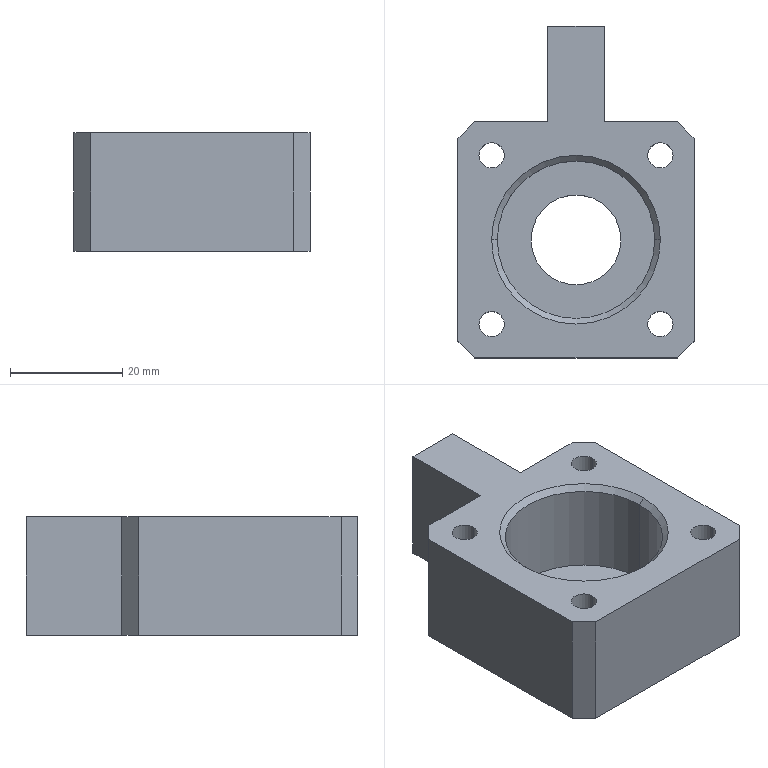Part | SolidWorks | features ICE 4, Chamfer 2, HoleWzd 2, Extrusion 1 | 1 solid | 49 faces | box 42 x 59 x 21 mm | volume 26880 mm3 | cylinder 24 | plane 19 | cone 6 | commonest cylinder face diameters 4.5 x8 8 x8 2.5 x4 16 x2 28 x2
STEP:
#1=CARTESIAN_POINT('',(-14.,23.25,20.));
#2=VERTEX_POINT('',#1);
#3=CARTESIAN_POINT('',(14.,23.25,20.));
#4=VERTEX_POINT('',#3);
#5=CARTESIAN_POINT('',(0.,23.25,20.));
#6=DIRECTION('',(0.,0.,1.));
#7=DIRECTION('',(1.,0.,0.));
#8=AXIS2_PLACEMENT_3D('',#5,#6,#7);
#9=CIRCLE('',#8,14.);
#10=EDGE_CURVE('',#2,#4,#9,.T.);
#11=ORIENTED_EDGE('',*,*,#10,.F.);
#12=CARTESIAN_POINT('',(-15.,23.25,21.));
#13=VERTEX_POINT('',#12);
#14=CARTESIAN_POINT('',(-14.,23.25,20.));
#15=DIRECTION('',(-0.7071,0.,0.7071));
#16=VECTOR('',#15,1000.);
#17=LINE('',#14,#16);
#18=EDGE_CURVE('',#2,#13,#17,.T.);
#19=ORIENTED_EDGE('',*,*,#18,.T.);
#20=CARTESIAN_POINT('',(15.,23.25,21.));
#21=VERTEX_POINT('',#20);
#22=CARTESIAN_POINT('',(0.,23.25,21.));
#23=DIRECTION('',(0.,0.,-1.));
#24=DIRECTION('',(1.,0.,0.));
#25=AXIS2_PLACEMENT_3D('',#22,#23,#24);
#26=CIRCLE('',#25,15.);
#27=EDGE_CURVE('',#21,#13,#26,.T.);
#28=ORIENTED_EDGE('',*,*,#27,.F.);
#29=CARTESIAN_POINT('',(14.,23.25,20.));
#30=DIRECTION('',(0.7071,0.,0.7071));
#31=VECTOR('',#30,1000.);
#32=LINE('',#29,#31);
#33=EDGE_CURVE('',#4,#21,#32,.T.);
#34=ORIENTED_EDGE('',*,*,#33,.F.);
#35=EDGE_LOOP('',(#11,#19,#28,#34));
#36=FACE_OUTER_BOUND('',#35,.T.);
#37=CARTESIAN_POINT('',(0.,23.25,20.));
#38=DIRECTION('',(0.,0.,1.));
#39=DIRECTION('',(1.,0.,0.));
#40=AXIS2_PLACEMENT_3D('',#37,#38,#39);
#41=CONICAL_SURFACE('',#40,14.,0.7854);
#42=ADVANCED_FACE('',(#36),#41,.F.);
#43=CARTESIAN_POINT('',(1.25,57.75,7.));
#44=VERTEX_POINT('',#43);
#45=CARTESIAN_POINT('',(-1.25,57.75,7.));
#46=VERTEX_POINT('',#45);
#47=CARTESIAN_POINT('',(0.,57.75,7.));
#48=DIRECTION('',(0.,0.,-1.));
#49=DIRECTION('',(-1.,0.,0.));
#50=AXIS2_PLACEMENT_3D('',#47,#48,#49);
#51=CIRCLE('',#50,1.25);
#52=EDGE_CURVE('',#44,#46,#51,.T.);
#53=ORIENTED_EDGE('',*,*,#52,.F.);
#54=CARTESIAN_POINT('',(1.25,57.75,0.));
#55=VERTEX_POINT('',#54);
#56=CARTESIAN_POINT('',(1.25,57.75,0.));
#57=DIRECTION('',(0.,0.,-1.));
#58=VECTOR('',#57,1000.);
#59=LINE('',#56,#58);
#60=EDGE_CURVE('',#44,#55,#59,.T.);
#61=ORIENTED_EDGE('',*,*,#60,.T.);
#62=CARTESIAN_POINT('',(-1.25,57.75,0.));
#63=VERTEX_POINT('',#62);
#64=CARTESIAN_POINT('',(0.,57.75,0.));
#65=DIRECTION('',(0.,0.,-1.));
#66=DIRECTION('',(-1.,0.,0.));
#67=AXIS2_PLACEMENT_3D('',#64,#65,#66);
#68=CIRCLE('',#67,1.25);
#69=EDGE_CURVE('',#55,#63,#68,.T.);
#70=ORIENTED_EDGE('',*,*,#69,.T.);
#71=CARTESIAN_POINT('',(-1.25,57.75,0.));
#72=DIRECTION('',(0.,0.,-1.));
#73=VECTOR('',#72,1000.);
#74=LINE('',#71,#73);
#75=EDGE_CURVE('',#46,#63,#74,.T.);
#76=ORIENTED_EDGE('',*,*,#75,.F.);
#77=EDGE_LOOP('',(#53,#61,#70,#76));
#78=FACE_OUTER_BOUND('',#77,.T.);
#79=CARTESIAN_POINT('',(0.,57.75,0.));
#80=DIRECTION('',(0.,0.,-1.));
#81=DIRECTION('',(-1.,0.,0.));
#82=AXIS2_PLACEMENT_3D('',#79,#80,#81);
#83=CYLINDRICAL_SURFACE('',#82,1.25);
#84=ADVANCED_FACE('',(#78),#83,.F.);
#85=CARTESIAN_POINT('',(0.,57.75,7.751));
#86=VERTEX_POINT('',#85);
#87=CARTESIAN_POINT('',(-1.25,57.75,7.));
#88=DIRECTION('',(-0.8572,0.,-0.515));
#89=VECTOR('',#88,1000.);
#90=LINE('',#87,#89);
#91=EDGE_CURVE('',#86,#46,#90,.T.);
#92=ORIENTED_EDGE('',*,*,#91,.F.);
#93=CARTESIAN_POINT('',(1.25,57.75,7.));
#94=DIRECTION('',(0.8572,0.,-0.515));
#95=VECTOR('',#94,1000.);
#96=LINE('',#93,#95);
#97=EDGE_CURVE('',#86,#44,#96,.T.);
#98=ORIENTED_EDGE('',*,*,#97,.T.);
#99=ORIENTED_EDGE('',*,*,#52,.T.);
#100=EDGE_LOOP('',(#92,#98,#99));
#101=FACE_OUTER_BOUND('',#100,.T.);
#102=CARTESIAN_POINT('',(0.,57.75,7.));
#103=DIRECTION('',(0.,0.,-1.));
#104=DIRECTION('',(-1.,0.,0.));
#105=AXIS2_PLACEMENT_3D('',#102,#103,#104);
#106=CONICAL_SURFACE('',#105,1.25,1.03);
#107=ADVANCED_FACE('',(#101),#106,.F.);
#108=CARTESIAN_POINT('',(1.25,39.25,7.));
#109=VERTEX_POINT('',#108);
#110=CARTESIAN_POINT('',(-1.25,39.25,7.));
#111=VERTEX_POINT('',#110);
#112=CARTESIAN_POINT('',(0.,39.25,7.));
#113=DIRECTION('',(0.,0.,-1.));
#114=DIRECTION('',(-1.,0.,0.));
#115=AXIS2_PLACEMENT_3D('',#112,#113,#114);
#116=CIRCLE('',#115,1.25);
#117=EDGE_CURVE('',#109,#111,#116,.T.);
#118=ORIENTED_EDGE('',*,*,#117,.F.);
#119=CARTESIAN_POINT('',(1.25,39.25,0.));
#120=VERTEX_POINT('',#119);
#121=CARTESIAN_POINT('',(1.25,39.25,0.));
#122=DIRECTION('',(0.,0.,-1.));
#123=VECTOR('',#122,1000.);
#124=LINE('',#121,#123);
#125=EDGE_CURVE('',#109,#120,#124,.T.);
#126=ORIENTED_EDGE('',*,*,#125,.T.);
#127=CARTESIAN_POINT('',(-1.25,39.25,0.));
#128=VERTEX_POINT('',#127);
#129=CARTESIAN_POINT('',(0.,39.25,0.));
#130=DIRECTION('',(0.,0.,-1.));
#131=DIRECTION('',(-1.,0.,0.));
#132=AXIS2_PLACEMENT_3D('',#129,#130,#131);
#133=CIRCLE('',#132,1.25);
#134=EDGE_CURVE('',#120,#128,#133,.T.);
#135=ORIENTED_EDGE('',*,*,#134,.T.);
#136=CARTESIAN_POINT('',(-1.25,39.25,0.));
#137=DIRECTION('',(0.,0.,-1.));
#138=VECTOR('',#137,1000.);
#139=LINE('',#136,#138);
#140=EDGE_CURVE('',#111,#128,#139,.T.);
#141=ORIENTED_EDGE('',*,*,#140,.F.);
#142=EDGE_LOOP('',(#118,#126,#135,#141));
#143=FACE_OUTER_BOUND('',#142,.T.);
#144=CARTESIAN_POINT('',(0.,39.25,0.));
#145=DIRECTION('',(0.,0.,-1.));
#146=DIRECTION('',(-1.,0.,0.));
#147=AXIS2_PLACEMENT_3D('',#144,#145,#146);
#148=CYLINDRICAL_SURFACE('',#147,1.25);
#149=ADVANCED_FACE('',(#143),#148,.F.);
#150=CARTESIAN_POINT('',(0.,39.25,7.751));
#151=VERTEX_POINT('',#150);
#152=CARTESIAN_POINT('',(-1.25,39.25,7.));
#153=DIRECTION('',(-0.8572,0.,-0.515));
#154=VECTOR('',#153,1000.);
#155=LINE('',#152,#154);
#156=EDGE_CURVE('',#151,#111,#155,.T.);
#157=ORIENTED_EDGE('',*,*,#156,.F.);
#158=CARTESIAN_POINT('',(1.25,39.25,7.));
#159=DIRECTION('',(0.8572,0.,-0.515));
#160=VECTOR('',#159,1000.);
#161=LINE('',#158,#160);
#162=EDGE_CURVE('',#151,#109,#161,.T.);
#163=ORIENTED_EDGE('',*,*,#162,.T.);
#164=ORIENTED_EDGE('',*,*,#117,.T.);
#165=EDGE_LOOP('',(#157,#163,#164));
#166=FACE_OUTER_BOUND('',#165,.T.);
#167=CARTESIAN_POINT('',(0.,39.25,7.));
#168=DIRECTION('',(0.,0.,-1.));
#169=DIRECTION('',(-1.,0.,0.));
#170=AXIS2_PLACEMENT_3D('',#167,#168,#169);
#171=CONICAL_SURFACE('',#170,1.25,1.03);
#172=ADVANCED_FACE('',(#166),#171,.F.);
#173=CARTESIAN_POINT('',(19.,38.25,4.6));
#174=VERTEX_POINT('',#173);
#175=CARTESIAN_POINT('',(11.,38.25,4.6));
#176=VERTEX_POINT('',#175);
#177=CARTESIAN_POINT('',(15.,38.25,4.6));
#178=DIRECTION('',(0.,0.,-1.));
#179=DIRECTION('',(-1.,0.,0.));
#180=AXIS2_PLACEMENT_3D('',#177,#178,#179);
#181=CIRCLE('',#180,4.);
#182=EDGE_CURVE('',#174,#176,#181,.T.);
#183=ORIENTED_EDGE('',*,*,#182,.F.);
#184=CARTESIAN_POINT('',(19.,38.25,0.));
#185=VERTEX_POINT('',#184);
#186=CARTESIAN_POINT('',(19.,38.25,0.));
#187=DIRECTION('',(0.,0.,-1.));
#188=VECTOR('',#187,1000.);
#189=LINE('',#186,#188);
#190=EDGE_CURVE('',#174,#185,#189,.T.);
#191=ORIENTED_EDGE('',*,*,#190,.T.);
#192=CARTESIAN_POINT('',(11.,38.25,0.));
#193=VERTEX_POINT('',#192);
#194=CARTESIAN_POINT('',(15.,38.25,0.));
#195=DIRECTION('',(0.,0.,-1.));
#196=DIRECTION('',(-1.,0.,0.));
#197=AXIS2_PLACEMENT_3D('',#194,#195,#196);
#198=CIRCLE('',#197,4.);
#199=EDGE_CURVE('',#185,#193,#198,.T.);
#200=ORIENTED_EDGE('',*,*,#199,.T.);
#201=CARTESIAN_POINT('',(11.,38.25,0.));
#202=DIRECTION('',(0.,0.,-1.));
#203=VECTOR('',#202,1000.);
#204=LINE('',#201,#203);
#205=EDGE_CURVE('',#176,#193,#204,.T.);
#206=ORIENTED_EDGE('',*,*,#205,.F.);
#207=EDGE_LOOP('',(#183,#191,#200,#206));
#208=FACE_OUTER_BOUND('',#207,.T.);
#209=CARTESIAN_POINT('',(15.,38.25,0.));
#210=DIRECTION('',(0.,0.,-1.));
#211=DIRECTION('',(-1.,0.,0.));
#212=AXIS2_PLACEMENT_3D('',#209,#210,#211);
#213=CYLINDRICAL_SURFACE('',#212,4.);
#214=ADVANCED_FACE('',(#208),#213,.F.);
#215=CARTESIAN_POINT('',(12.75,38.25,21.));
#216=VERTEX_POINT('',#215);
#217=CARTESIAN_POINT('',(17.25,38.25,21.));
#218=VERTEX_POINT('',#217);
#219=CARTESIAN_POINT('',(15.,38.25,21.));
#220=DIRECTION('',(0.,0.,1.));
#221=DIRECTION('',(1.,0.,0.));
#222=AXIS2_PLACEMENT_3D('',#219,#220,#221);
#223=CIRCLE('',#222,2.25);
#224=EDGE_CURVE('',#216,#218,#223,.T.);
#225=ORIENTED_EDGE('',*,*,#224,.T.);
#226=CARTESIAN_POINT('',(17.25,38.25,4.6));
#227=VERTEX_POINT('',#226);
#228=CARTESIAN_POINT('',(17.25,38.25,0.));
#229=DIRECTION('',(0.,0.,-1.));
#230=VECTOR('',#229,1000.);
#231=LINE('',#228,#230);
#232=EDGE_CURVE('',#218,#227,#231,.T.);
#233=ORIENTED_EDGE('',*,*,#232,.T.);
#234=CARTESIAN_POINT('',(12.75,38.25,4.6));
#235=VERTEX_POINT('',#234);
#236=CARTESIAN_POINT('',(15.,38.25,4.6));
#237=DIRECTION('',(0.,0.,-1.));
#238=DIRECTION('',(-1.,0.,0.));
#239=AXIS2_PLACEMENT_3D('',#236,#237,#238);
#240=CIRCLE('',#239,2.25);
#241=EDGE_CURVE('',#227,#235,#240,.T.);
#242=ORIENTED_EDGE('',*,*,#241,.T.);
#243=CARTESIAN_POINT('',(12.75,38.25,0.));
#244=DIRECTION('',(0.,0.,-1.));
#245=VECTOR('',#244,1000.);
#246=LINE('',#243,#245);
#247=EDGE_CURVE('',#216,#235,#246,.T.);
#248=ORIENTED_EDGE('',*,*,#247,.F.);
#249=EDGE_LOOP('',(#225,#233,#242,#248));
#250=FACE_OUTER_BOUND('',#249,.T.);
#251=CARTESIAN_POINT('',(15.,38.25,0.));
#252=DIRECTION('',(0.,0.,-1.));
#253=DIRECTION('',(-1.,0.,0.));
#254=AXIS2_PLACEMENT_3D('',#251,#252,#253);
#255=CYLINDRICAL_SURFACE('',#254,2.25);
#256=ADVANCED_FACE('',(#250),#255,.F.);
#257=CARTESIAN_POINT('',(-11.,38.25,4.6));
#258=VERTEX_POINT('',#257);
#259=CARTESIAN_POINT('',(-19.,38.25,4.6));
#260=VERTEX_POINT('',#259);
#261=CARTESIAN_POINT('',(-15.,38.25,4.6));
#262=DIRECTION('',(0.,0.,-1.));
#263=DIRECTION('',(-1.,0.,0.));
#264=AXIS2_PLACEMENT_3D('',#261,#262,#263);
#265=CIRCLE('',#264,4.);
#266=EDGE_CURVE('',#258,#260,#265,.T.);
#267=ORIENTED_EDGE('',*,*,#266,.F.);
#268=CARTESIAN_POINT('',(-11.,38.25,0.));
#269=VERTEX_POINT('',#268);
#270=CARTESIAN_POINT('',(-11.,38.25,0.));
#271=DIRECTION('',(0.,0.,-1.));
#272=VECTOR('',#271,1000.);
#273=LINE('',#270,#272);
#274=EDGE_CURVE('',#258,#269,#273,.T.);
#275=ORIENTED_EDGE('',*,*,#274,.T.);
#276=CARTESIAN_POINT('',(-19.,38.25,0.));
#277=VERTEX_POINT('',#276);
#278=CARTESIAN_POINT('',(-15.,38.25,0.));
#279=DIRECTION('',(0.,0.,-1.));
#280=DIRECTION('',(-1.,0.,0.));
#281=AXIS2_PLACEMENT_3D('',#278,#279,#280);
#282=CIRCLE('',#281,4.);
#283=EDGE_CURVE('',#269,#277,#282,.T.);
#284=ORIENTED_EDGE('',*,*,#283,.T.);
#285=CARTESIAN_POINT('',(-19.,38.25,0.));
#286=DIRECTION('',(0.,0.,-1.));
#287=VECTOR('',#286,1000.);
#288=LINE('',#285,#287);
#289=EDGE_CURVE('',#260,#277,#288,.T.);
#290=ORIENTED_EDGE('',*,*,#289,.F.);
#291=EDGE_LOOP('',(#267,#275,#284,#290));
#292=FACE_OUTER_BOUND('',#291,.T.);
#293=CARTESIAN_POINT('',(-15.,38.25,0.));
#294=DIRECTION('',(0.,0.,-1.));
#295=DIRECTION('',(-1.,0.,0.));
#296=AXIS2_PLACEMENT_3D('',#293,#294,#295);
#297=CYLINDRICAL_SURFACE('',#296,4.);
#298=ADVANCED_FACE('',(#292),#297,.F.);
#299=CARTESIAN_POINT('',(-17.25,38.25,21.));
#300=VERTEX_POINT('',#299);
#301=CARTESIAN_POINT('',(-12.75,38.25,21.));
#302=VERTEX_POINT('',#301);
#303=CARTESIAN_POINT('',(-15.,38.25,21.));
#304=DIRECTION('',(0.,0.,1.));
#305=DIRECTION('',(1.,0.,0.));
#306=AXIS2_PLACEMENT_3D('',#303,#304,#305);
#307=CIRCLE('',#306,2.25);
#308=EDGE_CURVE('',#300,#302,#307,.T.);
#309=ORIENTED_EDGE('',*,*,#308,.T.);
#310=CARTESIAN_POINT('',(-12.75,38.25,4.6));
#311=VERTEX_POINT('',#310);
#312=CARTESIAN_POINT('',(-12.75,38.25,0.));
#313=DIRECTION('',(0.,0.,-1.));
#314=VECTOR('',#313,1000.);
#315=LINE('',#312,#314);
#316=EDGE_CURVE('',#302,#311,#315,.T.);
#317=ORIENTED_EDGE('',*,*,#316,.T.);
#318=CARTESIAN_POINT('',(-17.25,38.25,4.6));
#319=VERTEX_POINT('',#318);
#320=CARTESIAN_POINT('',(-15.,38.25,4.6));
#321=DIRECTION('',(0.,0.,-1.));
#322=DIRECTION('',(-1.,0.,0.));
#323=AXIS2_PLACEMENT_3D('',#320,#321,#322);
#324=CIRCLE('',#323,2.25);
#325=EDGE_CURVE('',#311,#319,#324,.T.);
#326=ORIENTED_EDGE('',*,*,#325,.T.);
#327=CARTESIAN_POINT('',(-17.25,38.25,0.));
#328=DIRECTION('',(0.,0.,-1.));
#329=VECTOR('',#328,1000.);
#330=LINE('',#327,#329);
#331=EDGE_CURVE('',#300,#319,#330,.T.);
#332=ORIENTED_EDGE('',*,*,#331,.F.);
#333=EDGE_LOOP('',(#309,#317,#326,#332));
#334=FACE_OUTER_BOUND('',#333,.T.);
#335=CARTESIAN_POINT('',(-15.,38.25,0.));
#336=DIRECTION('',(0.,0.,-1.));
#337=DIRECTION('',(-1.,0.,0.));
#338=AXIS2_PLACEMENT_3D('',#335,#336,#337);
#339=CYLINDRICAL_SURFACE('',#338,2.25);
#340=ADVANCED_FACE('',(#334),#339,.F.);
#341=CARTESIAN_POINT('',(-11.,8.25,4.6));
#342=VERTEX_POINT('',#341);
#343=CARTESIAN_POINT('',(-19.,8.25,4.6));
#344=VERTEX_POINT('',#343);
#345=CARTESIAN_POINT('',(-15.,8.25,4.6));
#346=DIRECTION('',(0.,0.,-1.));
#347=DIRECTION('',(-1.,0.,0.));
#348=AXIS2_PLACEMENT_3D('',#345,#346,#347);
#349=CIRCLE('',#348,4.);
#350=EDGE_CURVE('',#342,#344,#349,.T.);
#351=ORIENTED_EDGE('',*,*,#350,.F.);
#352=CARTESIAN_POINT('',(-11.,8.25,0.));
#353=VERTEX_POINT('',#352);
#354=CARTESIAN_POINT('',(-11.,8.25,0.));
#355=DIRECTION('',(0.,0.,-1.));
#356=VECTOR('',#355,1000.);
#357=LINE('',#354,#356);
#358=EDGE_CURVE('',#342,#353,#357,.T.);
#359=ORIENTED_EDGE('',*,*,#358,.T.);
#360=CARTESIAN_POINT('',(-19.,8.25,0.));
#361=VERTEX_POINT('',#360);
#362=CARTESIAN_POINT('',(-15.,8.25,0.));
#363=DIRECTION('',(0.,0.,-1.));
#364=DIRECTION('',(-1.,0.,0.));
#365=AXIS2_PLACEMENT_3D('',#362,#363,#364);
#366=CIRCLE('',#365,4.);
#367=EDGE_CURVE('',#353,#361,#366,.T.);
#368=ORIENTED_EDGE('',*,*,#367,.T.);
#369=CARTESIAN_POINT('',(-19.,8.25,0.));
#370=DIRECTION('',(0.,0.,-1.));
#371=VECTOR('',#370,1000.);
#372=LINE('',#369,#371);
#373=EDGE_CURVE('',#344,#361,#372,.T.);
#374=ORIENTED_EDGE('',*,*,#373,.F.);
#375=EDGE_LOOP('',(#351,#359,#368,#374));
#376=FACE_OUTER_BOUND('',#375,.T.);
#377=CARTESIAN_POINT('',(-15.,8.25,0.));
#378=DIRECTION('',(0.,0.,-1.));
#379=DIRECTION('',(-1.,0.,0.));
#380=AXIS2_PLACEMENT_3D('',#377,#378,#379);
#381=CYLINDRICAL_SURFACE('',#380,4.);
#382=ADVANCED_FACE('',(#376),#381,.F.);
#383=CARTESIAN_POINT('',(-17.25,8.25,21.));
#384=VERTEX_POINT('',#383);
#385=CARTESIAN_POINT('',(-12.75,8.25,21.));
#386=VERTEX_POINT('',#385);
#387=CARTESIAN_POINT('',(-15.,8.25,21.));
#388=DIRECTION('',(0.,0.,1.));
#389=DIRECTION('',(1.,0.,0.));
#390=AXIS2_PLACEMENT_3D('',#387,#388,#389);
#391=CIRCLE('',#390,2.25);
#392=EDGE_CURVE('',#384,#386,#391,.T.);
#393=ORIENTED_EDGE('',*,*,#392,.T.);
#394=CARTESIAN_POINT('',(-12.75,8.25,4.6));
#395=VERTEX_POINT('',#394);
#396=CARTESIAN_POINT('',(-12.75,8.25,0.));
#397=DIRECTION('',(0.,0.,-1.));
#398=VECTOR('',#397,1000.);
#399=LINE('',#396,#398);
#400=EDGE_CURVE('',#386,#395,#399,.T.);
#401=ORIENTED_EDGE('',*,*,#400,.T.);
#402=CARTESIAN_POINT('',(-17.25,8.25,4.6));
#403=VERTEX_POINT('',#402);
#404=CARTESIAN_POINT('',(-15.,8.25,4.6));
#405=DIRECTION('',(0.,0.,-1.));
#406=DIRECTION('',(-1.,0.,0.));
#407=AXIS2_PLACEMENT_3D('',#404,#405,#406);
#408=CIRCLE('',#407,2.25);
#409=EDGE_CURVE('',#395,#403,#408,.T.);
#410=ORIENTED_EDGE('',*,*,#409,.T.);
#411=CARTESIAN_POINT('',(-17.25,8.25,0.));
#412=DIRECTION('',(0.,0.,-1.));
#413=VECTOR('',#412,1000.);
#414=LINE('',#411,#413);
#415=EDGE_CURVE('',#384,#403,#414,.T.);
#416=ORIENTED_EDGE('',*,*,#415,.F.);
#417=EDGE_LOOP('',(#393,#401,#410,#416));
#418=FACE_OUTER_BOUND('',#417,.T.);
#419=CARTESIAN_POINT('',(-15.,8.25,0.));
#420=DIRECTION('',(0.,0.,-1.));
#421=DIRECTION('',(-1.,0.,0.));
#422=AXIS2_PLACEMENT_3D('',#419,#420,#421);
#423=CYLINDRICAL_SURFACE('',#422,2.25);
#424=ADVANCED_FACE('',(#418),#423,.F.);
#425=CARTESIAN_POINT('',(19.,8.25,4.6));
#426=VERTEX_POINT('',#425);
#427=CARTESIAN_POINT('',(11.,8.25,4.6));
#428=VERTEX_POINT('',#427);
#429=CARTESIAN_POINT('',(15.,8.25,4.6));
#430=DIRECTION('',(0.,0.,-1.));
#431=DIRECTION('',(-1.,0.,0.));
#432=AXIS2_PLACEMENT_3D('',#429,#430,#431);
#433=CIRCLE('',#432,4.);
#434=EDGE_CURVE('',#426,#428,#433,.T.);
#435=ORIENTED_EDGE('',*,*,#434,.F.);
#436=CARTESIAN_POINT('',(19.,8.25,0.));
#437=VERTEX_POINT('',#436);
#438=CARTESIAN_POINT('',(19.,8.25,0.));
#439=DIRECTION('',(0.,0.,-1.));
#440=VECTOR('',#439,1000.);
#441=LINE('',#438,#440);
#442=EDGE_CURVE('',#426,#437,#441,.T.);
#443=ORIENTED_EDGE('',*,*,#442,.T.);
#444=CARTESIAN_POINT('',(11.,8.25,0.));
#445=VERTEX_POINT('',#444);
#446=CARTESIAN_POINT('',(15.,8.25,0.));
#447=DIRECTION('',(0.,0.,-1.));
#448=DIRECTION('',(-1.,0.,0.));
#449=AXIS2_PLACEMENT_3D('',#446,#447,#448);
#450=CIRCLE('',#449,4.);
#451=EDGE_CURVE('',#437,#445,#450,.T.);
#452=ORIENTED_EDGE('',*,*,#451,.T.);
#453=CARTESIAN_POINT('',(11.,8.25,0.));
#454=DIRECTION('',(0.,0.,-1.));
#455=VECTOR('',#454,1000.);
#456=LINE('',#453,#455);
#457=EDGE_CURVE('',#428,#445,#456,.T.);
#458=ORIENTED_EDGE('',*,*,#457,.F.);
#459=EDGE_LOOP('',(#435,#443,#452,#458));
#460=FACE_OUTER_BOUND('',#459,.T.);
#461=CARTESIAN_POINT('',(15.,8.25,0.));
#462=DIRECTION('',(0.,0.,-1.));
#463=DIRECTION('',(-1.,0.,0.));
#464=AXIS2_PLACEMENT_3D('',#461,#462,#463);
#465=CYLINDRICAL_SURFACE('',#464,4.);
#466=ADVANCED_FACE('',(#460),#465,.F.);
#467=CARTESIAN_POINT('',(12.75,8.25,21.));
#468=VERTEX_POINT('',#467);
#469=CARTESIAN_POINT('',(17.25,8.25,21.));
#470=VERTEX_POINT('',#469);
#471=CARTESIAN_POINT('',(15.,8.25,21.));
#472=DIRECTION('',(0.,0.,1.));
#473=DIRECTION('',(1.,0.,0.));
#474=AXIS2_PLACEMENT_3D('',#471,#472,#473);
#475=CIRCLE('',#474,2.25);
#476=EDGE_CURVE('',#468,#470,#475,.T.);
#477=ORIENTED_EDGE('',*,*,#476,.T.);
#478=CARTESIAN_POINT('',(17.25,8.25,4.6));
#479=VERTEX_POINT('',#478);
#480=CARTESIAN_POINT('',(17.25,8.25,0.));
#481=DIRECTION('',(0.,0.,-1.));
#482=VECTOR('',#481,1000.);
#483=LINE('',#480,#482);
#484=EDGE_CURVE('',#470,#479,#483,.T.);
#485=ORIENTED_EDGE('',*,*,#484,.T.);
#486=CARTESIAN_POINT('',(12.75,8.25,4.6));
#487=VERTEX_POINT('',#486);
#488=CARTESIAN_POINT('',(15.,8.25,4.6));
#489=DIRECTION('',(0.,0.,-1.));
#490=DIRECTION('',(-1.,0.,0.));
#491=AXIS2_PLACEMENT_3D('',#488,#489,#490);
#492=CIRCLE('',#491,2.25);
#493=EDGE_CURVE('',#479,#487,#492,.T.);
#494=ORIENTED_EDGE('',*,*,#493,.T.);
#495=CARTESIAN_POINT('',(12.75,8.25,0.));
#496=DIRECTION('',(0.,0.,-1.));
#497=VECTOR('',#496,1000.);
#498=LINE('',#495,#497);
#499=EDGE_CURVE('',#468,#487,#498,.T.);
#500=ORIENTED_EDGE('',*,*,#499,.F.);
#501=EDGE_LOOP('',(#477,#485,#494,#500));
#502=FACE_OUTER_BOUND('',#501,.T.);
#503=CARTESIAN_POINT('',(15.,8.25,0.));
#504=DIRECTION('',(0.,0.,-1.));
#505=DIRECTION('',(-1.,0.,0.));
#506=AXIS2_PLACEMENT_3D('',#503,#504,#505);
#507=CYLINDRICAL_SURFACE('',#506,2.25);
#508=ADVANCED_FACE('',(#502),#507,.F.);
#509=CARTESIAN_POINT('',(-8.,23.25,0.));
#510=VERTEX_POINT('',#509);
#511=CARTESIAN_POINT('',(8.,23.25,0.));
#512=VERTEX_POINT('',#511);
#513=CARTESIAN_POINT('',(0.,23.25,0.));
#514=DIRECTION('',(0.,0.,1.));
#515=DIRECTION('',(1.,0.,0.));
#516=AXIS2_PLACEMENT_3D('',#513,#514,#515);
#517=CIRCLE('',#516,8.);
#518=EDGE_CURVE('',#510,#512,#517,.T.);
#519=ORIENTED_EDGE('',*,*,#518,.F.);
#520=CARTESIAN_POINT('',(-8.,23.25,4.));
#521=VERTEX_POINT('',#520);
#522=CARTESIAN_POINT('',(-8.,23.25,0.));
#523=DIRECTION('',(0.,0.,1.));
#524=VECTOR('',#523,1000.);
#525=LINE('',#522,#524);
#526=EDGE_CURVE('',#510,#521,#525,.T.);
#527=ORIENTED_EDGE('',*,*,#526,.T.);
#528=CARTESIAN_POINT('',(8.,23.25,4.));
#529=VERTEX_POINT('',#528);
#530=CARTESIAN_POINT('',(0.,23.25,4.));
#531=DIRECTION('',(0.,0.,1.));
#532=DIRECTION('',(1.,0.,0.));
#533=AXIS2_PLACEMENT_3D('',#530,#531,#532);
#534=CIRCLE('',#533,8.);
#535=EDGE_CURVE('',#521,#529,#534,.T.);
#536=ORIENTED_EDGE('',*,*,#535,.T.);
#537=CARTESIAN_POINT('',(8.,23.25,0.));
#538=DIRECTION('',(0.,0.,1.));
#539=VECTOR('',#538,1000.);
#540=LINE('',#537,#539);
#541=EDGE_CURVE('',#512,#529,#540,.T.);
#542=ORIENTED_EDGE('',*,*,#541,.F.);
#543=EDGE_LOOP('',(#519,#527,#536,#542));
#544=FACE_OUTER_BOUND('',#543,.T.);
#545=CARTESIAN_POINT('',(0.,23.25,0.));
#546=DIRECTION('',(0.,0.,1.));
#547=DIRECTION('',(1.,0.,0.));
#548=AXIS2_PLACEMENT_3D('',#545,#546,#547);
#549=CYLINDRICAL_SURFACE('',#548,8.);
#550=ADVANCED_FACE('',(#544),#549,.F.);
#551=CARTESIAN_POINT('',(-14.,23.25,4.));
#552=VERTEX_POINT('',#551);
#553=CARTESIAN_POINT('',(14.,23.25,4.));
#554=VERTEX_POINT('',#553);
#555=CARTESIAN_POINT('',(0.,23.25,4.));
#556=DIRECTION('',(0.,0.,1.));
#557=DIRECTION('',(1.,0.,0.));
#558=AXIS2_PLACEMENT_3D('',#555,#556,#557);
#559=CIRCLE('',#558,14.);
#560=EDGE_CURVE('',#552,#554,#559,.T.);
#561=ORIENTED_EDGE('',*,*,#560,.F.);
#562=CARTESIAN_POINT('',(-14.,23.25,4.));
#563=DIRECTION('',(0.,0.,1.));
#564=VECTOR('',#563,1000.);
#565=LINE('',#562,#564);
#566=EDGE_CURVE('',#552,#2,#565,.T.);
#567=ORIENTED_EDGE('',*,*,#566,.T.);
#568=ORIENTED_EDGE('',*,*,#10,.T.);
#569=CARTESIAN_POINT('',(14.,23.25,4.));
#570=DIRECTION('',(0.,0.,1.));
#571=VECTOR('',#570,1000.);
#572=LINE('',#569,#571);
#573=EDGE_CURVE('',#554,#4,#572,.T.);
#574=ORIENTED_EDGE('',*,*,#573,.F.);
#575=EDGE_LOOP('',(#561,#567,#568,#574));
#576=FACE_OUTER_BOUND('',#575,.T.);
#577=CARTESIAN_POINT('',(0.,23.25,4.));
#578=DIRECTION('',(0.,0.,1.));
#579=DIRECTION('',(1.,0.,0.));
#580=AXIS2_PLACEMENT_3D('',#577,#578,#579);
#581=CYLINDRICAL_SURFACE('',#580,14.);
#582=ADVANCED_FACE('',(#576),#581,.F.);
#583=CARTESIAN_POINT('',(5.,44.25,21.));
#584=VERTEX_POINT('',#583);
#585=CARTESIAN_POINT('',(5.,44.25,0.));
#586=VERTEX_POINT('',#585);
#587=CARTESIAN_POINT('',(5.,44.25,21.));
#588=DIRECTION('',(0.,0.,-1.));
#589=VECTOR('',#588,1000.);
#590=LINE('',#587,#589);
#591=EDGE_CURVE('',#584,#586,#590,.T.);
#592=ORIENTED_EDGE('',*,*,#591,.F.);
#593=CARTESIAN_POINT('',(18.,44.25,21.));
#594=VERTEX_POINT('',#593);
#595=CARTESIAN_POINT('',(18.,44.25,21.));
#596=DIRECTION('',(-1.,0.,0.));
#597=VECTOR('',#596,1000.);
#598=LINE('',#595,#597);
#599=EDGE_CURVE('',#594,#584,#598,.T.);
#600=ORIENTED_EDGE('',*,*,#599,.F.);
#601=CARTESIAN_POINT('',(18.,44.25,0.));
#602=VERTEX_POINT('',#601);
#603=CARTESIAN_POINT('',(18.,44.25,12.));
#604=DIRECTION('',(0.,0.,-1.));
#605=VECTOR('',#604,1000.);
#606=LINE('',#603,#605);
#607=EDGE_CURVE('',#594,#602,#606,.T.);
#608=ORIENTED_EDGE('',*,*,#607,.T.);
#609=CARTESIAN_POINT('',(-21.,44.25,0.));
#610=DIRECTION('',(-1.,0.,0.));
#611=VECTOR('',#610,1000.);
#612=LINE('',#609,#611);
#613=EDGE_CURVE('',#602,#586,#612,.T.);
#614=ORIENTED_EDGE('',*,*,#613,.T.);
#615=EDGE_LOOP('',(#592,#600,#608,#614));
#616=FACE_OUTER_BOUND('',#615,.T.);
#617=CARTESIAN_POINT('',(-21.,44.25,12.));
#618=DIRECTION('',(0.,-1.,0.));
#619=DIRECTION('',(0.,0.,-1.));
#620=AXIS2_PLACEMENT_3D('',#617,#618,#619);
#621=PLANE('',#620);
#622=ADVANCED_FACE('',(#616),#621,.F.);
#623=CARTESIAN_POINT('',(21.,41.25,0.));
#624=VERTEX_POINT('',#623);
#625=CARTESIAN_POINT('',(21.,41.25,21.));
#626=VERTEX_POINT('',#625);
#627=CARTESIAN_POINT('',(21.,41.25,12.));
#628=DIRECTION('',(0.,0.,1.));
#629=VECTOR('',#628,1000.);
#630=LINE('',#627,#629);
#631=EDGE_CURVE('',#624,#626,#630,.T.);
#632=ORIENTED_EDGE('',*,*,#631,.T.);
#633=CARTESIAN_POINT('',(21.,5.25,21.));
#634=VERTEX_POINT('',#633);
#635=CARTESIAN_POINT('',(21.,5.25,21.));
#636=DIRECTION('',(0.,1.,0.));
#637=VECTOR('',#636,1000.);
#638=LINE('',#635,#637);
#639=EDGE_CURVE('',#634,#626,#638,.T.);
#640=ORIENTED_EDGE('',*,*,#639,.F.);
#641=CARTESIAN_POINT('',(21.,5.25,0.));
#642=VERTEX_POINT('',#641);
#643=CARTESIAN_POINT('',(21.,5.25,12.));
#644=DIRECTION('',(0.,0.,-1.));
#645=VECTOR('',#644,1000.);
#646=LINE('',#643,#645);
#647=EDGE_CURVE('',#634,#642,#646,.T.);
#648=ORIENTED_EDGE('',*,*,#647,.T.);
#649=CARTESIAN_POINT('',(21.,2.25,0.));
#650=DIRECTION('',(0.,1.,0.));
#651=VECTOR('',#650,1000.);
#652=LINE('',#649,#651);
#653=EDGE_CURVE('',#642,#624,#652,.T.);
#654=ORIENTED_EDGE('',*,*,#653,.T.);
#655=EDGE_LOOP('',(#632,#640,#648,#654));
#656=FACE_OUTER_BOUND('',#655,.T.);
#657=CARTESIAN_POINT('',(21.,2.25,12.));
#658=DIRECTION('',(-1.,0.,0.));
#659=DIRECTION('',(0.,0.,1.));
#660=AXIS2_PLACEMENT_3D('',#657,#658,#659);
#661=PLANE('',#660);
#662=ADVANCED_FACE('',(#656),#661,.F.);
#663=CARTESIAN_POINT('',(-5.,44.25,21.));
#664=VERTEX_POINT('',#663);
#665=CARTESIAN_POINT('',(-18.,44.25,21.));
#666=VERTEX_POINT('',#665);
#667=CARTESIAN_POINT('',(18.,44.25,21.));
#668=DIRECTION('',(-1.,0.,0.));
#669=VECTOR('',#668,1000.);
#670=LINE('',#667,#669);
#671=EDGE_CURVE('',#664,#666,#670,.T.);
#672=ORIENTED_EDGE('',*,*,#671,.F.);
#673=CARTESIAN_POINT('',(-5.,44.25,0.));
#674=VERTEX_POINT('',#673);
#675=CARTESIAN_POINT('',(-5.,44.25,21.));
#676=DIRECTION('',(0.,0.,-1.));
#677=VECTOR('',#676,1000.);
#678=LINE('',#675,#677);
#679=EDGE_CURVE('',#664,#674,#678,.T.);
#680=ORIENTED_EDGE('',*,*,#679,.T.);
#681=CARTESIAN_POINT('',(-18.,44.25,0.));
#682=VERTEX_POINT('',#681);
#683=CARTESIAN_POINT('',(-21.,44.25,0.));
#684=DIRECTION('',(-1.,0.,0.));
#685=VECTOR('',#684,1000.);
#686=LINE('',#683,#685);
#687=EDGE_CURVE('',#674,#682,#686,.T.);
#688=ORIENTED_EDGE('',*,*,#687,.T.);
#689=CARTESIAN_POINT('',(-18.,44.25,12.));
#690=DIRECTION('',(0.,0.,1.));
#691=VECTOR('',#690,1000.);
#692=LINE('',#689,#691);
#693=EDGE_CURVE('',#682,#666,#692,.T.);
#694=ORIENTED_EDGE('',*,*,#693,.T.);
#695=EDGE_LOOP('',(#672,#680,#688,#694));
#696=FACE_OUTER_BOUND('',#695,.T.);
#697=CARTESIAN_POINT('',(-21.,44.25,12.));
#698=DIRECTION('',(0.,-1.,0.));
#699=DIRECTION('',(0.,0.,-1.));
#700=AXIS2_PLACEMENT_3D('',#697,#698,#699);
#701=PLANE('',#700);
#702=ADVANCED_FACE('',(#696),#701,.F.);
#703=CARTESIAN_POINT('',(-21.,41.25,0.));
#704=VERTEX_POINT('',#703);
#705=CARTESIAN_POINT('',(-21.,5.25,0.));
#706=VERTEX_POINT('',#705);
#707=CARTESIAN_POINT('',(-21.,2.25,0.));
#708=DIRECTION('',(0.,-1.,0.));
#709=VECTOR('',#708,1000.);
#710=LINE('',#707,#709);
#711=EDGE_CURVE('',#704,#706,#710,.T.);
#712=ORIENTED_EDGE('',*,*,#711,.T.);
#713=CARTESIAN_POINT('',(-21.,5.25,21.));
#714=VERTEX_POINT('',#713);
#715=CARTESIAN_POINT('',(-21.,5.25,12.));
#716=DIRECTION('',(0.,0.,1.));
#717=VECTOR('',#716,1000.);
#718=LINE('',#715,#717);
#719=EDGE_CURVE('',#706,#714,#718,.T.);
#720=ORIENTED_EDGE('',*,*,#719,.T.);
#721=CARTESIAN_POINT('',(-21.,41.25,21.));
#722=VERTEX_POINT('',#721);
#723=CARTESIAN_POINT('',(-21.,41.25,21.));
#724=DIRECTION('',(0.,-1.,0.));
#725=VECTOR('',#724,1000.);
#726=LINE('',#723,#725);
#727=EDGE_CURVE('',#722,#714,#726,.T.);
#728=ORIENTED_EDGE('',*,*,#727,.F.);
#729=CARTESIAN_POINT('',(-21.,41.25,12.));
#730=DIRECTION('',(0.,0.,-1.));
#731=VECTOR('',#730,1000.);
#732=LINE('',#729,#731);
#733=EDGE_CURVE('',#722,#704,#732,.T.);
#734=ORIENTED_EDGE('',*,*,#733,.T.);
#735=EDGE_LOOP('',(#712,#720,#728,#734));
#736=FACE_OUTER_BOUND('',#735,.T.);
#737=CARTESIAN_POINT('',(-21.,2.25,12.));
#738=DIRECTION('',(1.,0.,0.));
#739=DIRECTION('',(0.,0.,-1.));
#740=AXIS2_PLACEMENT_3D('',#737,#738,#739);
#741=PLANE('',#740);
#742=ADVANCED_FACE('',(#736),#741,.F.);
#743=CARTESIAN_POINT('',(-18.,2.25,0.));
#744=VERTEX_POINT('',#743);
#745=CARTESIAN_POINT('',(18.,2.25,0.));
#746=VERTEX_POINT('',#745);
#747=CARTESIAN_POINT('',(-21.,2.25,0.));
#748=DIRECTION('',(1.,0.,0.));
#749=VECTOR('',#748,1000.);
#750=LINE('',#747,#749);
#751=EDGE_CURVE('',#744,#746,#750,.T.);
#752=ORIENTED_EDGE('',*,*,#751,.T.);
#753=CARTESIAN_POINT('',(18.,2.25,21.));
#754=VERTEX_POINT('',#753);
#755=CARTESIAN_POINT('',(18.,2.25,12.));
#756=DIRECTION('',(0.,0.,1.));
#757=VECTOR('',#756,1000.);
#758=LINE('',#755,#757);
#759=EDGE_CURVE('',#746,#754,#758,.T.);
#760=ORIENTED_EDGE('',*,*,#759,.T.);
#761=CARTESIAN_POINT('',(-18.,2.25,21.));
#762=VERTEX_POINT('',#761);
#763=CARTESIAN_POINT('',(-18.,2.25,21.));
#764=DIRECTION('',(1.,0.,0.));
#765=VECTOR('',#764,1000.);
#766=LINE('',#763,#765);
#767=EDGE_CURVE('',#762,#754,#766,.T.);
#768=ORIENTED_EDGE('',*,*,#767,.F.);
#769=CARTESIAN_POINT('',(-18.,2.25,12.));
#770=DIRECTION('',(0.,0.,-1.));
#771=VECTOR('',#770,1000.);
#772=LINE('',#769,#771);
#773=EDGE_CURVE('',#762,#744,#772,.T.);
#774=ORIENTED_EDGE('',*,*,#773,.T.);
#775=EDGE_LOOP('',(#752,#760,#768,#774));
#776=FACE_OUTER_BOUND('',#775,.T.);
#777=CARTESIAN_POINT('',(-21.,2.25,12.));
#778=DIRECTION('',(0.,1.,0.));
#779=DIRECTION('',(0.,0.,1.));
#780=AXIS2_PLACEMENT_3D('',#777,#778,#779);
#781=PLANE('',#780);
#782=ADVANCED_FACE('',(#776),#781,.F.);
#783=CARTESIAN_POINT('',(0.,57.75,0.));
#784=DIRECTION('',(0.,0.,-1.));
#785=DIRECTION('',(-1.,0.,0.));
#786=AXIS2_PLACEMENT_3D('',#783,#784,#785);
#787=CIRCLE('',#786,1.25);
#788=EDGE_CURVE('',#63,#55,#787,.T.);
#789=ORIENTED_EDGE('',*,*,#788,.F.);
#790=ORIENTED_EDGE('',*,*,#69,.F.);
#791=EDGE_LOOP('',(#789,#790));
#792=FACE_BOUND('',#791,.T.);
#793=CARTESIAN_POINT('',(0.,39.25,0.));
#794=DIRECTION('',(0.,0.,-1.));
#795=DIRECTION('',(-1.,0.,0.));
#796=AXIS2_PLACEMENT_3D('',#793,#794,#795);
#797=CIRCLE('',#796,1.25);
#798=EDGE_CURVE('',#128,#120,#797,.T.);
#799=ORIENTED_EDGE('',*,*,#798,.F.);
#800=ORIENTED_EDGE('',*,*,#134,.F.);
#801=EDGE_LOOP('',(#799,#800));
#802=FACE_BOUND('',#801,.T.);
#803=CARTESIAN_POINT('',(15.,38.25,0.));
#804=DIRECTION('',(0.,0.,-1.));
#805=DIRECTION('',(-1.,0.,0.));
#806=AXIS2_PLACEMENT_3D('',#803,#804,#805);
#807=CIRCLE('',#806,4.);
#808=EDGE_CURVE('',#193,#185,#807,.T.);
#809=ORIENTED_EDGE('',*,*,#808,.F.);
#810=ORIENTED_EDGE('',*,*,#199,.F.);
#811=EDGE_LOOP('',(#809,#810));
#812=FACE_BOUND('',#811,.T.);
#813=CARTESIAN_POINT('',(-15.,38.25,0.));
#814=DIRECTION('',(0.,0.,-1.));
#815=DIRECTION('',(-1.,0.,0.));
#816=AXIS2_PLACEMENT_3D('',#813,#814,#815);
#817=CIRCLE('',#816,4.);
#818=EDGE_CURVE('',#277,#269,#817,.T.);
#819=ORIENTED_EDGE('',*,*,#818,.F.);
#820=ORIENTED_EDGE('',*,*,#283,.F.);
#821=EDGE_LOOP('',(#819,#820));
#822=FACE_BOUND('',#821,.T.);
#823=CARTESIAN_POINT('',(-15.,8.25,0.));
#824=DIRECTION('',(0.,0.,-1.));
#825=DIRECTION('',(-1.,0.,0.));
#826=AXIS2_PLACEMENT_3D('',#823,#824,#825);
#827=CIRCLE('',#826,4.);
#828=EDGE_CURVE('',#361,#353,#827,.T.);
#829=ORIENTED_EDGE('',*,*,#828,.F.);
#830=ORIENTED_EDGE('',*,*,#367,.F.);
#831=EDGE_LOOP('',(#829,#830));
#832=FACE_BOUND('',#831,.T.);
#833=CARTESIAN_POINT('',(15.,8.25,0.));
#834=DIRECTION('',(0.,0.,-1.));
#835=DIRECTION('',(-1.,0.,0.));
#836=AXIS2_PLACEMENT_3D('',#833,#834,#835);
#837=CIRCLE('',#836,4.);
#838=EDGE_CURVE('',#445,#437,#837,.T.);
#839=ORIENTED_EDGE('',*,*,#838,.F.);
#840=ORIENTED_EDGE('',*,*,#451,.F.);
#841=EDGE_LOOP('',(#839,#840));
#842=FACE_BOUND('',#841,.T.);
#843=CARTESIAN_POINT('',(0.,23.25,0.));
#844=DIRECTION('',(0.,0.,1.));
#845=DIRECTION('',(1.,0.,0.));
#846=AXIS2_PLACEMENT_3D('',#843,#844,#845);
#847=CIRCLE('',#846,8.);
#848=EDGE_CURVE('',#512,#510,#847,.T.);
#849=ORIENTED_EDGE('',*,*,#848,.T.);
#850=ORIENTED_EDGE('',*,*,#518,.T.);
#851=EDGE_LOOP('',(#849,#850));
#852=FACE_BOUND('',#851,.T.);
#853=ORIENTED_EDGE('',*,*,#653,.F.);
#854=CARTESIAN_POINT('',(7.875,-7.875,0.));
#855=DIRECTION('',(-0.7071,-0.7071,0.));
#856=VECTOR('',#855,1000.);
#857=LINE('',#854,#856);
#858=EDGE_CURVE('',#642,#746,#857,.T.);
#859=ORIENTED_EDGE('',*,*,#858,.T.);
#860=ORIENTED_EDGE('',*,*,#751,.F.);
#861=CARTESIAN_POINT('',(-7.875,-7.875,0.));
#862=DIRECTION('',(-0.7071,0.7071,0.));
#863=VECTOR('',#862,1000.);
#864=LINE('',#861,#863);
#865=EDGE_CURVE('',#744,#706,#864,.T.);
#866=ORIENTED_EDGE('',*,*,#865,.T.);
#867=ORIENTED_EDGE('',*,*,#711,.F.);
#868=CARTESIAN_POINT('',(-31.125,31.125,0.));
#869=DIRECTION('',(0.7071,0.7071,0.));
#870=VECTOR('',#869,1000.);
#871=LINE('',#868,#870);
#872=EDGE_CURVE('',#704,#682,#871,.T.);
#873=ORIENTED_EDGE('',*,*,#872,.T.);
#874=ORIENTED_EDGE('',*,*,#687,.F.);
#875=CARTESIAN_POINT('',(-5.,61.25,0.));
#876=VERTEX_POINT('',#875);
#877=CARTESIAN_POINT('',(-5.,61.25,0.));
#878=DIRECTION('',(0.,1.,0.));
#879=VECTOR('',#878,1000.);
#880=LINE('',#877,#879);
#881=EDGE_CURVE('',#674,#876,#880,.T.);
#882=ORIENTED_EDGE('',*,*,#881,.T.);
#883=CARTESIAN_POINT('',(5.,61.25,0.));
#884=VERTEX_POINT('',#883);
#885=CARTESIAN_POINT('',(5.,61.25,0.));
#886=DIRECTION('',(1.,0.,0.));
#887=VECTOR('',#886,1000.);
#888=LINE('',#885,#887);
#889=EDGE_CURVE('',#876,#884,#888,.T.);
#890=ORIENTED_EDGE('',*,*,#889,.T.);
#891=CARTESIAN_POINT('',(5.,44.25,0.));
#892=DIRECTION('',(0.,-1.,0.));
#893=VECTOR('',#892,1000.);
#894=LINE('',#891,#893);
#895=EDGE_CURVE('',#884,#586,#894,.T.);
#896=ORIENTED_EDGE('',*,*,#895,.T.);
#897=ORIENTED_EDGE('',*,*,#613,.F.);
#898=CARTESIAN_POINT('',(31.125,31.125,0.));
#899=DIRECTION('',(0.7071,-0.7071,0.));
#900=VECTOR('',#899,1000.);
#901=LINE('',#898,#900);
#902=EDGE_CURVE('',#602,#624,#901,.T.);
#903=ORIENTED_EDGE('',*,*,#902,.T.);
#904=EDGE_LOOP('',(#853,#859,#860,#866,#867,#873,#874,#882,#890,#896,#897,#903));
#905=FACE_OUTER_BOUND('',#904,.T.);
#906=CARTESIAN_POINT('',(0.,0.,0.));
#907=DIRECTION('',(0.,0.,-1.));
#908=DIRECTION('',(-1.,0.,0.));
#909=AXIS2_PLACEMENT_3D('',#906,#907,#908);
#910=PLANE('',#909);
#911=ADVANCED_FACE('',(#792,#802,#812,#822,#832,#842,#852,#905),#910,.T.);
#912=ORIENTED_EDGE('',*,*,#566,.F.);
#913=CARTESIAN_POINT('',(0.,23.25,4.));
#914=DIRECTION('',(0.,0.,1.));
#915=DIRECTION('',(1.,0.,0.));
#916=AXIS2_PLACEMENT_3D('',#913,#914,#915);
#917=CIRCLE('',#916,14.);
#918=EDGE_CURVE('',#554,#552,#917,.T.);
#919=ORIENTED_EDGE('',*,*,#918,.F.);
#920=ORIENTED_EDGE('',*,*,#573,.T.);
#921=CARTESIAN_POINT('',(0.,23.25,20.));
#922=DIRECTION('',(0.,0.,1.));
#923=DIRECTION('',(1.,0.,0.));
#924=AXIS2_PLACEMENT_3D('',#921,#922,#923);
#925=CIRCLE('',#924,14.);
#926=EDGE_CURVE('',#4,#2,#925,.T.);
#927=ORIENTED_EDGE('',*,*,#926,.T.);
#928=EDGE_LOOP('',(#912,#919,#920,#927));
#929=FACE_OUTER_BOUND('',#928,.T.);
#930=CARTESIAN_POINT('',(0.,23.25,4.));
#931=DIRECTION('',(0.,0.,1.));
#932=DIRECTION('',(1.,0.,0.));
#933=AXIS2_PLACEMENT_3D('',#930,#931,#932);
#934=CYLINDRICAL_SURFACE('',#933,14.);
#935=ADVANCED_FACE('',(#929),#934,.F.);
#936=CARTESIAN_POINT('',(0.,23.25,4.));
#937=DIRECTION('',(0.,0.,1.));
#938=DIRECTION('',(1.,0.,0.));
#939=AXIS2_PLACEMENT_3D('',#936,#937,#938);
#940=CIRCLE('',#939,8.);
#941=EDGE_CURVE('',#529,#521,#940,.T.);
#942=ORIENTED_EDGE('',*,*,#941,.F.);
#943=ORIENTED_EDGE('',*,*,#535,.F.);
#944=EDGE_LOOP('',(#942,#943));
#945=FACE_BOUND('',#944,.T.);
#946=ORIENTED_EDGE('',*,*,#918,.T.);
#947=ORIENTED_EDGE('',*,*,#560,.T.);
#948=EDGE_LOOP('',(#946,#947));
#949=FACE_OUTER_BOUND('',#948,.T.);
#950=CARTESIAN_POINT('',(0.,23.25,4.));
#951=DIRECTION('',(0.,0.,1.));
#952=DIRECTION('',(1.,0.,0.));
#953=AXIS2_PLACEMENT_3D('',#950,#951,#952);
#954=PLANE('',#953);
#955=ADVANCED_FACE('',(#945,#949),#954,.T.);
#956=ORIENTED_EDGE('',*,*,#526,.F.);
#957=ORIENTED_EDGE('',*,*,#848,.F.);
#958=ORIENTED_EDGE('',*,*,#541,.T.);
#959=ORIENTED_EDGE('',*,*,#941,.T.);
#960=EDGE_LOOP('',(#956,#957,#958,#959));
#961=FACE_OUTER_BOUND('',#960,.T.);
#962=CARTESIAN_POINT('',(0.,23.25,0.));
#963=DIRECTION('',(0.,0.,1.));
#964=DIRECTION('',(1.,0.,0.));
#965=AXIS2_PLACEMENT_3D('',#962,#963,#964);
#966=CYLINDRICAL_SURFACE('',#965,8.);
#967=ADVANCED_FACE('',(#961),#966,.F.);
#968=ORIENTED_EDGE('',*,*,#647,.F.);
#969=CARTESIAN_POINT('',(18.,2.25,21.));
#970=DIRECTION('',(0.7071,0.7071,0.));
#971=VECTOR('',#970,1000.);
#972=LINE('',#969,#971);
#973=EDGE_CURVE('',#754,#634,#972,.T.);
#974=ORIENTED_EDGE('',*,*,#973,.F.);
#975=ORIENTED_EDGE('',*,*,#759,.F.);
#976=ORIENTED_EDGE('',*,*,#858,.F.);
#977=EDGE_LOOP('',(#968,#974,#975,#976));
#978=FACE_OUTER_BOUND('',#977,.T.);
#979=CARTESIAN_POINT('',(21.,5.25,12.));
#980=DIRECTION('',(-0.7071,0.7071,0.));
#981=DIRECTION('',(0.,0.,-1.));
#982=AXIS2_PLACEMENT_3D('',#979,#980,#981);
#983=PLANE('',#982);
#984=ADVANCED_FACE('',(#978),#983,.F.);
#985=ORIENTED_EDGE('',*,*,#773,.F.);
#986=CARTESIAN_POINT('',(-21.,5.25,21.));
#987=DIRECTION('',(0.7071,-0.7071,0.));
#988=VECTOR('',#987,1000.);
#989=LINE('',#986,#988);
#990=EDGE_CURVE('',#714,#762,#989,.T.);
#991=ORIENTED_EDGE('',*,*,#990,.F.);
#992=ORIENTED_EDGE('',*,*,#719,.F.);
#993=ORIENTED_EDGE('',*,*,#865,.F.);
#994=EDGE_LOOP('',(#985,#991,#992,#993));
#995=FACE_OUTER_BOUND('',#994,.T.);
#996=CARTESIAN_POINT('',(-18.,2.25,12.));
#997=DIRECTION('',(0.7071,0.7071,0.));
#998=DIRECTION('',(0.,0.,-1.));
#999=AXIS2_PLACEMENT_3D('',#996,#997,#998);
#1000=PLANE('',#999);
#1001=ADVANCED_FACE('',(#995),#1000,.F.);
#1002=ORIENTED_EDGE('',*,*,#733,.F.);
#1003=CARTESIAN_POINT('',(-18.,44.25,21.));
#1004=DIRECTION('',(-0.7071,-0.7071,0.));
#1005=VECTOR('',#1004,1000.);
#1006=LINE('',#1003,#1005);
#1007=EDGE_CURVE('',#666,#722,#1006,.T.);
#1008=ORIENTED_EDGE('',*,*,#1007,.F.);
#1009=ORIENTED_EDGE('',*,*,#693,.F.);
#1010=ORIENTED_EDGE('',*,*,#872,.F.);
#1011=EDGE_LOOP('',(#1002,#1008,#1009,#1010));
#1012=FACE_OUTER_BOUND('',#1011,.T.);
#1013=CARTESIAN_POINT('',(-21.,41.25,12.));
#1014=DIRECTION('',(0.7071,-0.7071,0.));
#1015=DIRECTION('',(0.,0.,-1.));
#1016=AXIS2_PLACEMENT_3D('',#1013,#1014,#1015);
#1017=PLANE('',#1016);
#1018=ADVANCED_FACE('',(#1012),#1017,.F.);
#1019=ORIENTED_EDGE('',*,*,#607,.F.);
#1020=CARTESIAN_POINT('',(21.,41.25,21.));
#1021=DIRECTION('',(-0.7071,0.7071,0.));
#1022=VECTOR('',#1021,1000.);
#1023=LINE('',#1020,#1022);
#1024=EDGE_CURVE('',#626,#594,#1023,.T.);
#1025=ORIENTED_EDGE('',*,*,#1024,.F.);
#1026=ORIENTED_EDGE('',*,*,#631,.F.);
#1027=ORIENTED_EDGE('',*,*,#902,.F.);
#1028=EDGE_LOOP('',(#1019,#1025,#1026,#1027));
#1029=FACE_OUTER_BOUND('',#1028,.T.);
#1030=CARTESIAN_POINT('',(18.,44.25,12.));
#1031=DIRECTION('',(-0.7071,-0.7071,0.));
#1032=DIRECTION('',(0.,0.,-1.));
#1033=AXIS2_PLACEMENT_3D('',#1030,#1031,#1032);
#1034=PLANE('',#1033);
#1035=ADVANCED_FACE('',(#1029),#1034,.F.);
#1036=ORIENTED_EDGE('',*,*,#484,.F.);
#1037=CARTESIAN_POINT('',(15.,8.25,21.));
#1038=DIRECTION('',(0.,0.,1.));
#1039=DIRECTION('',(1.,0.,0.));
#1040=AXIS2_PLACEMENT_3D('',#1037,#1038,#1039);
#1041=CIRCLE('',#1040,2.25);
#1042=EDGE_CURVE('',#470,#468,#1041,.T.);
#1043=ORIENTED_EDGE('',*,*,#1042,.T.);
#1044=ORIENTED_EDGE('',*,*,#499,.T.);
#1045=CARTESIAN_POINT('',(15.,8.25,4.6));
#1046=DIRECTION('',(0.,0.,-1.));
#1047=DIRECTION('',(-1.,0.,0.));
#1048=AXIS2_PLACEMENT_3D('',#1045,#1046,#1047);
#1049=CIRCLE('',#1048,2.25);
#1050=EDGE_CURVE('',#487,#479,#1049,.T.);
#1051=ORIENTED_EDGE('',*,*,#1050,.T.);
#1052=EDGE_LOOP('',(#1036,#1043,#1044,#1051));
#1053=FACE_OUTER_BOUND('',#1052,.T.);
#1054=CARTESIAN_POINT('',(15.,8.25,0.));
#1055=DIRECTION('',(0.,0.,-1.));
#1056=DIRECTION('',(-1.,0.,0.));
#1057=AXIS2_PLACEMENT_3D('',#1054,#1055,#1056);
#1058=CYLINDRICAL_SURFACE('',#1057,2.25);
#1059=ADVANCED_FACE('',(#1053),#1058,.F.);
#1060=ORIENTED_EDGE('',*,*,#1050,.F.);
#1061=ORIENTED_EDGE('',*,*,#493,.F.);
#1062=EDGE_LOOP('',(#1060,#1061));
#1063=FACE_BOUND('',#1062,.T.);
#1064=CARTESIAN_POINT('',(15.,8.25,4.6));
#1065=DIRECTION('',(0.,0.,-1.));
#1066=DIRECTION('',(-1.,0.,0.));
#1067=AXIS2_PLACEMENT_3D('',#1064,#1065,#1066);
#1068=CIRCLE('',#1067,4.);
#1069=EDGE_CURVE('',#428,#426,#1068,.T.);
#1070=ORIENTED_EDGE('',*,*,#1069,.T.);
#1071=ORIENTED_EDGE('',*,*,#434,.T.);
#1072=EDGE_LOOP('',(#1070,#1071));
#1073=FACE_OUTER_BOUND('',#1072,.T.);
#1074=CARTESIAN_POINT('',(17.25,8.25,4.6));
#1075=DIRECTION('',(0.,0.,1.));
#1076=DIRECTION('',(1.,0.,0.));
#1077=AXIS2_PLACEMENT_3D('',#1074,#1075,#1076);
#1078=PLANE('',#1077);
#1079=ADVANCED_FACE('',(#1063,#1073),#1078,.F.);
#1080=ORIENTED_EDGE('',*,*,#442,.F.);
#1081=ORIENTED_EDGE('',*,*,#1069,.F.);
#1082=ORIENTED_EDGE('',*,*,#457,.T.);
#1083=ORIENTED_EDGE('',*,*,#838,.T.);
#1084=EDGE_LOOP('',(#1080,#1081,#1082,#1083));
#1085=FACE_OUTER_BOUND('',#1084,.T.);
#1086=CARTESIAN_POINT('',(15.,8.25,0.));
#1087=DIRECTION('',(0.,0.,-1.));
#1088=DIRECTION('',(-1.,0.,0.));
#1089=AXIS2_PLACEMENT_3D('',#1086,#1087,#1088);
#1090=CYLINDRICAL_SURFACE('',#1089,4.);
#1091=ADVANCED_FACE('',(#1085),#1090,.F.);
#1092=ORIENTED_EDGE('',*,*,#400,.F.);
#1093=CARTESIAN_POINT('',(-15.,8.25,21.));
#1094=DIRECTION('',(0.,0.,1.));
#1095=DIRECTION('',(1.,0.,0.));
#1096=AXIS2_PLACEMENT_3D('',#1093,#1094,#1095);
#1097=CIRCLE('',#1096,2.25);
#1098=EDGE_CURVE('',#386,#384,#1097,.T.);
#1099=ORIENTED_EDGE('',*,*,#1098,.T.);
#1100=ORIENTED_EDGE('',*,*,#415,.T.);
#1101=CARTESIAN_POINT('',(-15.,8.25,4.6));
#1102=DIRECTION('',(0.,0.,-1.));
#1103=DIRECTION('',(-1.,0.,0.));
#1104=AXIS2_PLACEMENT_3D('',#1101,#1102,#1103);
#1105=CIRCLE('',#1104,2.25);
#1106=EDGE_CURVE('',#403,#395,#1105,.T.);
#1107=ORIENTED_EDGE('',*,*,#1106,.T.);
#1108=EDGE_LOOP('',(#1092,#1099,#1100,#1107));
#1109=FACE_OUTER_BOUND('',#1108,.T.);
#1110=CARTESIAN_POINT('',(-15.,8.25,0.));
#1111=DIRECTION('',(0.,0.,-1.));
#1112=DIRECTION('',(-1.,0.,0.));
#1113=AXIS2_PLACEMENT_3D('',#1110,#1111,#1112);
#1114=CYLINDRICAL_SURFACE('',#1113,2.25);
#1115=ADVANCED_FACE('',(#1109),#1114,.F.);
#1116=ORIENTED_EDGE('',*,*,#1106,.F.);
#1117=ORIENTED_EDGE('',*,*,#409,.F.);
#1118=EDGE_LOOP('',(#1116,#1117));
#1119=FACE_BOUND('',#1118,.T.);
#1120=CARTESIAN_POINT('',(-15.,8.25,4.6));
#1121=DIRECTION('',(0.,0.,-1.));
#1122=DIRECTION('',(-1.,0.,0.));
#1123=AXIS2_PLACEMENT_3D('',#1120,#1121,#1122);
#1124=CIRCLE('',#1123,4.);
#1125=EDGE_CURVE('',#344,#342,#1124,.T.);
#1126=ORIENTED_EDGE('',*,*,#1125,.T.);
#1127=ORIENTED_EDGE('',*,*,#350,.T.);
#1128=EDGE_LOOP('',(#1126,#1127));
#1129=FACE_OUTER_BOUND('',#1128,.T.);
#1130=CARTESIAN_POINT('',(-12.75,8.25,4.6));
#1131=DIRECTION('',(0.,0.,1.));
#1132=DIRECTION('',(1.,0.,0.));
#1133=AXIS2_PLACEMENT_3D('',#1130,#1131,#1132);
#1134=PLANE('',#1133);
#1135=ADVANCED_FACE('',(#1119,#1129),#1134,.F.);
#1136=ORIENTED_EDGE('',*,*,#358,.F.);
#1137=ORIENTED_EDGE('',*,*,#1125,.F.);
#1138=ORIENTED_EDGE('',*,*,#373,.T.);
#1139=ORIENTED_EDGE('',*,*,#828,.T.);
#1140=EDGE_LOOP('',(#1136,#1137,#1138,#1139));
#1141=FACE_OUTER_BOUND('',#1140,.T.);
#1142=CARTESIAN_POINT('',(-15.,8.25,0.));
#1143=DIRECTION('',(0.,0.,-1.));
#1144=DIRECTION('',(-1.,0.,0.));
#1145=AXIS2_PLACEMENT_3D('',#1142,#1143,#1144);
#1146=CYLINDRICAL_SURFACE('',#1145,4.);
#1147=ADVANCED_FACE('',(#1141),#1146,.F.);
#1148=ORIENTED_EDGE('',*,*,#316,.F.);
#1149=CARTESIAN_POINT('',(-15.,38.25,21.));
#1150=DIRECTION('',(0.,0.,1.));
#1151=DIRECTION('',(1.,0.,0.));
#1152=AXIS2_PLACEMENT_3D('',#1149,#1150,#1151);
#1153=CIRCLE('',#1152,2.25);
#1154=EDGE_CURVE('',#302,#300,#1153,.T.);
#1155=ORIENTED_EDGE('',*,*,#1154,.T.);
#1156=ORIENTED_EDGE('',*,*,#331,.T.);
#1157=CARTESIAN_POINT('',(-15.,38.25,4.6));
#1158=DIRECTION('',(0.,0.,-1.));
#1159=DIRECTION('',(-1.,0.,0.));
#1160=AXIS2_PLACEMENT_3D('',#1157,#1158,#1159);
#1161=CIRCLE('',#1160,2.25);
#1162=EDGE_CURVE('',#319,#311,#1161,.T.);
#1163=ORIENTED_EDGE('',*,*,#1162,.T.);
#1164=EDGE_LOOP('',(#1148,#1155,#1156,#1163));
#1165=FACE_OUTER_BOUND('',#1164,.T.);
#1166=CARTESIAN_POINT('',(-15.,38.25,0.));
#1167=DIRECTION('',(0.,0.,-1.));
#1168=DIRECTION('',(-1.,0.,0.));
#1169=AXIS2_PLACEMENT_3D('',#1166,#1167,#1168);
#1170=CYLINDRICAL_SURFACE('',#1169,2.25);
#1171=ADVANCED_FACE('',(#1165),#1170,.F.);
#1172=ORIENTED_EDGE('',*,*,#1162,.F.);
#1173=ORIENTED_EDGE('',*,*,#325,.F.);
#1174=EDGE_LOOP('',(#1172,#1173));
#1175=FACE_BOUND('',#1174,.T.);
#1176=CARTESIAN_POINT('',(-15.,38.25,4.6));
#1177=DIRECTION('',(0.,0.,-1.));
#1178=DIRECTION('',(-1.,0.,0.));
#1179=AXIS2_PLACEMENT_3D('',#1176,#1177,#1178);
#1180=CIRCLE('',#1179,4.);
#1181=EDGE_CURVE('',#260,#258,#1180,.T.);
#1182=ORIENTED_EDGE('',*,*,#1181,.T.);
#1183=ORIENTED_EDGE('',*,*,#266,.T.);
#1184=EDGE_LOOP('',(#1182,#1183));
#1185=FACE_OUTER_BOUND('',#1184,.T.);
#1186=CARTESIAN_POINT('',(-12.75,38.25,4.6));
#1187=DIRECTION('',(0.,0.,1.));
#1188=DIRECTION('',(1.,0.,0.));
#1189=AXIS2_PLACEMENT_3D('',#1186,#1187,#1188);
#1190=PLANE('',#1189);
#1191=ADVANCED_FACE('',(#1175,#1185),#1190,.F.);
#1192=ORIENTED_EDGE('',*,*,#274,.F.);
#1193=ORIENTED_EDGE('',*,*,#1181,.F.);
#1194=ORIENTED_EDGE('',*,*,#289,.T.);
#1195=ORIENTED_EDGE('',*,*,#818,.T.);
#1196=EDGE_LOOP('',(#1192,#1193,#1194,#1195));
#1197=FACE_OUTER_BOUND('',#1196,.T.);
#1198=CARTESIAN_POINT('',(-15.,38.25,0.));
#1199=DIRECTION('',(0.,0.,-1.));
#1200=DIRECTION('',(-1.,0.,0.));
#1201=AXIS2_PLACEMENT_3D('',#1198,#1199,#1200);
#1202=CYLINDRICAL_SURFACE('',#1201,4.);
#1203=ADVANCED_FACE('',(#1197),#1202,.F.);
#1204=ORIENTED_EDGE('',*,*,#232,.F.);
#1205=CARTESIAN_POINT('',(15.,38.25,21.));
#1206=DIRECTION('',(0.,0.,1.));
#1207=DIRECTION('',(1.,0.,0.));
#1208=AXIS2_PLACEMENT_3D('',#1205,#1206,#1207);
#1209=CIRCLE('',#1208,2.25);
#1210=EDGE_CURVE('',#218,#216,#1209,.T.);
#1211=ORIENTED_EDGE('',*,*,#1210,.T.);
#1212=ORIENTED_EDGE('',*,*,#247,.T.);
#1213=CARTESIAN_POINT('',(15.,38.25,4.6));
#1214=DIRECTION('',(0.,0.,-1.));
#1215=DIRECTION('',(-1.,0.,0.));
#1216=AXIS2_PLACEMENT_3D('',#1213,#1214,#1215);
#1217=CIRCLE('',#1216,2.25);
#1218=EDGE_CURVE('',#235,#227,#1217,.T.);
#1219=ORIENTED_EDGE('',*,*,#1218,.T.);
#1220=EDGE_LOOP('',(#1204,#1211,#1212,#1219));
#1221=FACE_OUTER_BOUND('',#1220,.T.);
#1222=CARTESIAN_POINT('',(15.,38.25,0.));
#1223=DIRECTION('',(0.,0.,-1.));
#1224=DIRECTION('',(-1.,0.,0.));
#1225=AXIS2_PLACEMENT_3D('',#1222,#1223,#1224);
#1226=CYLINDRICAL_SURFACE('',#1225,2.25);
#1227=ADVANCED_FACE('',(#1221),#1226,.F.);
#1228=ORIENTED_EDGE('',*,*,#1218,.F.);
#1229=ORIENTED_EDGE('',*,*,#241,.F.);
#1230=EDGE_LOOP('',(#1228,#1229));
#1231=FACE_BOUND('',#1230,.T.);
#1232=CARTESIAN_POINT('',(15.,38.25,4.6));
#1233=DIRECTION('',(0.,0.,-1.));
#1234=DIRECTION('',(-1.,0.,0.));
#1235=AXIS2_PLACEMENT_3D('',#1232,#1233,#1234);
#1236=CIRCLE('',#1235,4.);
#1237=EDGE_CURVE('',#176,#174,#1236,.T.);
#1238=ORIENTED_EDGE('',*,*,#1237,.T.);
#1239=ORIENTED_EDGE('',*,*,#182,.T.);
#1240=EDGE_LOOP('',(#1238,#1239));
#1241=FACE_OUTER_BOUND('',#1240,.T.);
#1242=CARTESIAN_POINT('',(17.25,38.25,4.6));
#1243=DIRECTION('',(0.,0.,1.));
#1244=DIRECTION('',(1.,0.,0.));
#1245=AXIS2_PLACEMENT_3D('',#1242,#1243,#1244);
#1246=PLANE('',#1245);
#1247=ADVANCED_FACE('',(#1231,#1241),#1246,.F.);
#1248=ORIENTED_EDGE('',*,*,#190,.F.);
#1249=ORIENTED_EDGE('',*,*,#1237,.F.);
#1250=ORIENTED_EDGE('',*,*,#205,.T.);
#1251=ORIENTED_EDGE('',*,*,#808,.T.);
#1252=EDGE_LOOP('',(#1248,#1249,#1250,#1251));
#1253=FACE_OUTER_BOUND('',#1252,.T.);
#1254=CARTESIAN_POINT('',(15.,38.25,0.));
#1255=DIRECTION('',(0.,0.,-1.));
#1256=DIRECTION('',(-1.,0.,0.));
#1257=AXIS2_PLACEMENT_3D('',#1254,#1255,#1256);
#1258=CYLINDRICAL_SURFACE('',#1257,4.);
#1259=ADVANCED_FACE('',(#1253),#1258,.F.);
#1260=ORIENTED_EDGE('',*,*,#27,.T.);
#1261=CARTESIAN_POINT('',(0.,23.25,21.));
#1262=DIRECTION('',(0.,0.,-1.));
#1263=DIRECTION('',(1.,0.,0.));
#1264=AXIS2_PLACEMENT_3D('',#1261,#1262,#1263);
#1265=CIRCLE('',#1264,15.);
#1266=EDGE_CURVE('',#13,#21,#1265,.T.);
#1267=ORIENTED_EDGE('',*,*,#1266,.T.);
#1268=EDGE_LOOP('',(#1260,#1267));
#1269=FACE_BOUND('',#1268,.T.);
#1270=ORIENTED_EDGE('',*,*,#476,.F.);
#1271=ORIENTED_EDGE('',*,*,#1042,.F.);
#1272=EDGE_LOOP('',(#1270,#1271));
#1273=FACE_BOUND('',#1272,.T.);
#1274=ORIENTED_EDGE('',*,*,#990,.T.);
#1275=ORIENTED_EDGE('',*,*,#767,.T.);
#1276=ORIENTED_EDGE('',*,*,#973,.T.);
#1277=ORIENTED_EDGE('',*,*,#639,.T.);
#1278=ORIENTED_EDGE('',*,*,#1024,.T.);
#1279=ORIENTED_EDGE('',*,*,#599,.T.);
#1280=CARTESIAN_POINT('',(5.,61.25,21.));
#1281=VERTEX_POINT('',#1280);
#1282=CARTESIAN_POINT('',(5.,44.25,21.));
#1283=DIRECTION('',(0.,-1.,0.));
#1284=VECTOR('',#1283,1000.);
#1285=LINE('',#1282,#1284);
#1286=EDGE_CURVE('',#1281,#584,#1285,.T.);
#1287=ORIENTED_EDGE('',*,*,#1286,.F.);
#1288=CARTESIAN_POINT('',(-5.,61.25,21.));
#1289=VERTEX_POINT('',#1288);
#1290=CARTESIAN_POINT('',(5.,61.25,21.));
#1291=DIRECTION('',(1.,0.,0.));
#1292=VECTOR('',#1291,1000.);
#1293=LINE('',#1290,#1292);
#1294=EDGE_CURVE('',#1289,#1281,#1293,.T.);
#1295=ORIENTED_EDGE('',*,*,#1294,.F.);
#1296=CARTESIAN_POINT('',(-5.,61.25,21.));
#1297=DIRECTION('',(0.,1.,0.));
#1298=VECTOR('',#1297,1000.);
#1299=LINE('',#1296,#1298);
#1300=EDGE_CURVE('',#664,#1289,#1299,.T.);
#1301=ORIENTED_EDGE('',*,*,#1300,.F.);
#1302=ORIENTED_EDGE('',*,*,#671,.T.);
#1303=ORIENTED_EDGE('',*,*,#1007,.T.);
#1304=ORIENTED_EDGE('',*,*,#727,.T.);
#1305=EDGE_LOOP('',(#1274,#1275,#1276,#1277,#1278,#1279,#1287,#1295,#1301,#1302,#1303,#1304));
#1306=FACE_OUTER_BOUND('',#1305,.T.);
#1307=ORIENTED_EDGE('',*,*,#308,.F.);
#1308=ORIENTED_EDGE('',*,*,#1154,.F.);
#1309=EDGE_LOOP('',(#1307,#1308));
#1310=FACE_BOUND('',#1309,.T.);
#1311=ORIENTED_EDGE('',*,*,#224,.F.);
#1312=ORIENTED_EDGE('',*,*,#1210,.F.);
#1313=EDGE_LOOP('',(#1311,#1312));
#1314=FACE_BOUND('',#1313,.T.);
#1315=ORIENTED_EDGE('',*,*,#392,.F.);
#1316=ORIENTED_EDGE('',*,*,#1098,.F.);
#1317=EDGE_LOOP('',(#1315,#1316));
#1318=FACE_BOUND('',#1317,.T.);
#1319=CARTESIAN_POINT('',(0.,0.,21.));
#1320=DIRECTION('',(0.,0.,1.));
#1321=DIRECTION('',(1.,0.,0.));
#1322=AXIS2_PLACEMENT_3D('',#1319,#1320,#1321);
#1323=PLANE('',#1322);
#1324=ADVANCED_FACE('',(#1269,#1273,#1306,#1310,#1314,#1318),#1323,.T.);
#1325=ORIENTED_EDGE('',*,*,#895,.F.);
#1326=CARTESIAN_POINT('',(5.,61.25,21.));
#1327=DIRECTION('',(0.,0.,-1.));
#1328=VECTOR('',#1327,1000.);
#1329=LINE('',#1326,#1328);
#1330=EDGE_CURVE('',#1281,#884,#1329,.T.);
#1331=ORIENTED_EDGE('',*,*,#1330,.F.);
#1332=ORIENTED_EDGE('',*,*,#1286,.T.);
#1333=ORIENTED_EDGE('',*,*,#591,.T.);
#1334=EDGE_LOOP('',(#1325,#1331,#1332,#1333));
#1335=FACE_OUTER_BOUND('',#1334,.T.);
#1336=CARTESIAN_POINT('',(5.,44.25,21.));
#1337=DIRECTION('',(1.,0.,0.));
#1338=DIRECTION('',(0.,0.,-1.));
#1339=AXIS2_PLACEMENT_3D('',#1336,#1337,#1338);
#1340=PLANE('',#1339);
#1341=ADVANCED_FACE('',(#1335),#1340,.T.);
#1342=ORIENTED_EDGE('',*,*,#889,.F.);
#1343=CARTESIAN_POINT('',(-5.,61.25,21.));
#1344=DIRECTION('',(0.,0.,-1.));
#1345=VECTOR('',#1344,1000.);
#1346=LINE('',#1343,#1345);
#1347=EDGE_CURVE('',#1289,#876,#1346,.T.);
#1348=ORIENTED_EDGE('',*,*,#1347,.F.);
#1349=ORIENTED_EDGE('',*,*,#1294,.T.);
#1350=ORIENTED_EDGE('',*,*,#1330,.T.);
#1351=EDGE_LOOP('',(#1342,#1348,#1349,#1350));
#1352=FACE_OUTER_BOUND('',#1351,.T.);
#1353=CARTESIAN_POINT('',(5.,61.25,21.));
#1354=DIRECTION('',(0.,1.,0.));
#1355=DIRECTION('',(0.,0.,1.));
#1356=AXIS2_PLACEMENT_3D('',#1353,#1354,#1355);
#1357=PLANE('',#1356);
#1358=ADVANCED_FACE('',(#1352),#1357,.T.);
#1359=ORIENTED_EDGE('',*,*,#881,.F.);
#1360=ORIENTED_EDGE('',*,*,#679,.F.);
#1361=ORIENTED_EDGE('',*,*,#1300,.T.);
#1362=ORIENTED_EDGE('',*,*,#1347,.T.);
#1363=EDGE_LOOP('',(#1359,#1360,#1361,#1362));
#1364=FACE_OUTER_BOUND('',#1363,.T.);
#1365=CARTESIAN_POINT('',(-5.,61.25,21.));
#1366=DIRECTION('',(-1.,0.,0.));
#1367=DIRECTION('',(0.,-1.,0.));
#1368=AXIS2_PLACEMENT_3D('',#1365,#1366,#1367);
#1369=PLANE('',#1368);
#1370=ADVANCED_FACE('',(#1364),#1369,.T.);
#1371=ORIENTED_EDGE('',*,*,#162,.F.);
#1372=ORIENTED_EDGE('',*,*,#156,.T.);
#1373=CARTESIAN_POINT('',(0.,39.25,7.));
#1374=DIRECTION('',(0.,0.,-1.));
#1375=DIRECTION('',(-1.,0.,0.));
#1376=AXIS2_PLACEMENT_3D('',#1373,#1374,#1375);
#1377=CIRCLE('',#1376,1.25);
#1378=EDGE_CURVE('',#111,#109,#1377,.T.);
#1379=ORIENTED_EDGE('',*,*,#1378,.T.);
#1380=EDGE_LOOP('',(#1371,#1372,#1379));
#1381=FACE_OUTER_BOUND('',#1380,.T.);
#1382=CARTESIAN_POINT('',(0.,39.25,7.));
#1383=DIRECTION('',(0.,0.,-1.));
#1384=DIRECTION('',(-1.,0.,0.));
#1385=AXIS2_PLACEMENT_3D('',#1382,#1383,#1384);
#1386=CONICAL_SURFACE('',#1385,1.25,1.03);
#1387=ADVANCED_FACE('',(#1381),#1386,.F.);
#1388=ORIENTED_EDGE('',*,*,#125,.F.);
#1389=ORIENTED_EDGE('',*,*,#1378,.F.);
#1390=ORIENTED_EDGE('',*,*,#140,.T.);
#1391=ORIENTED_EDGE('',*,*,#798,.T.);
#1392=EDGE_LOOP('',(#1388,#1389,#1390,#1391));
#1393=FACE_OUTER_BOUND('',#1392,.T.);
#1394=CARTESIAN_POINT('',(0.,39.25,0.));
#1395=DIRECTION('',(0.,0.,-1.));
#1396=DIRECTION('',(-1.,0.,0.));
#1397=AXIS2_PLACEMENT_3D('',#1394,#1395,#1396);
#1398=CYLINDRICAL_SURFACE('',#1397,1.25);
#1399=ADVANCED_FACE('',(#1393),#1398,.F.);
#1400=ORIENTED_EDGE('',*,*,#97,.F.);
#1401=ORIENTED_EDGE('',*,*,#91,.T.);
#1402=CARTESIAN_POINT('',(0.,57.75,7.));
#1403=DIRECTION('',(0.,0.,-1.));
#1404=DIRECTION('',(-1.,0.,0.));
#1405=AXIS2_PLACEMENT_3D('',#1402,#1403,#1404);
#1406=CIRCLE('',#1405,1.25);
#1407=EDGE_CURVE('',#46,#44,#1406,.T.);
#1408=ORIENTED_EDGE('',*,*,#1407,.T.);
#1409=EDGE_LOOP('',(#1400,#1401,#1408));
#1410=FACE_OUTER_BOUND('',#1409,.T.);
#1411=CARTESIAN_POINT('',(0.,57.75,7.));
#1412=DIRECTION('',(0.,0.,-1.));
#1413=DIRECTION('',(-1.,0.,0.));
#1414=AXIS2_PLACEMENT_3D('',#1411,#1412,#1413);
#1415=CONICAL_SURFACE('',#1414,1.25,1.03);
#1416=ADVANCED_FACE('',(#1410),#1415,.F.);
#1417=ORIENTED_EDGE('',*,*,#60,.F.);
#1418=ORIENTED_EDGE('',*,*,#1407,.F.);
#1419=ORIENTED_EDGE('',*,*,#75,.T.);
#1420=ORIENTED_EDGE('',*,*,#788,.T.);
#1421=EDGE_LOOP('',(#1417,#1418,#1419,#1420));
#1422=FACE_OUTER_BOUND('',#1421,.T.);
#1423=CARTESIAN_POINT('',(0.,57.75,0.));
#1424=DIRECTION('',(0.,0.,-1.));
#1425=DIRECTION('',(-1.,0.,0.));
#1426=AXIS2_PLACEMENT_3D('',#1423,#1424,#1425);
#1427=CYLINDRICAL_SURFACE('',#1426,1.25);
#1428=ADVANCED_FACE('',(#1422),#1427,.F.);
#1429=ORIENTED_EDGE('',*,*,#18,.F.);
#1430=ORIENTED_EDGE('',*,*,#926,.F.);
#1431=ORIENTED_EDGE('',*,*,#33,.T.);
#1432=ORIENTED_EDGE('',*,*,#1266,.F.);
#1433=EDGE_LOOP('',(#1429,#1430,#1431,#1432));
#1434=FACE_OUTER_BOUND('',#1433,.T.);
#1435=CARTESIAN_POINT('',(0.,23.25,20.));
#1436=DIRECTION('',(0.,0.,1.));
#1437=DIRECTION('',(1.,0.,0.));
#1438=AXIS2_PLACEMENT_3D('',#1435,#1436,#1437);
#1439=CONICAL_SURFACE('',#1438,14.,0.7854);
#1440=ADVANCED_FACE('',(#1434),#1439,.F.);
#1441=CLOSED_SHELL('',(#42,#84,#107,#149,#172,#214,#256,#298,#340,#382,#424,#466,#508,#550,#582,#622,#662,#702,#742,#782,#911,#935,#955,#967,#984,#1001,#1018,#1035,#1059,#1079,#1091,#1115,#1135,#1147,#1171,#1191,#1203,#1227,#1247,#1259,#1324,#1341,#1358,#1370,#1387,#1399,#1416,#1428,#1440));
#1442=MANIFOLD_SOLID_BREP('',#1441);
#1443=CARTESIAN_POINT('',(0.,0.,0.));
#1444=DIRECTION('',(0.,0.,1.));
#1445=DIRECTION('',(1.,0.,0.));
#1446=AXIS2_PLACEMENT_3D('',#1443,#1444,#1445);
#1447=(LENGTH_UNIT()NAMED_UNIT(*)SI_UNIT(.MILLI.,.METRE.));
#1448=UNCERTAINTY_MEASURE_WITH_UNIT(LENGTH_MEASURE(0.00001),#1447,'','');
#1449=(NAMED_UNIT(*)PLANE_ANGLE_UNIT()SI_UNIT($,.RADIAN.));
#1450=(NAMED_UNIT(*)SI_UNIT($,.STERADIAN.)SOLID_ANGLE_UNIT());
#1451=(GEOMETRIC_REPRESENTATION_CONTEXT(3)GLOBAL_UNCERTAINTY_ASSIGNED_CONTEXT((#1448))GLOBAL_UNIT_ASSIGNED_CONTEXT((#1447,#1449,#1450))REPRESENTATION_CONTEXT('',''));
#1452=ADVANCED_BREP_SHAPE_REPRESENTATION('',(#1442,#1446),#1451);